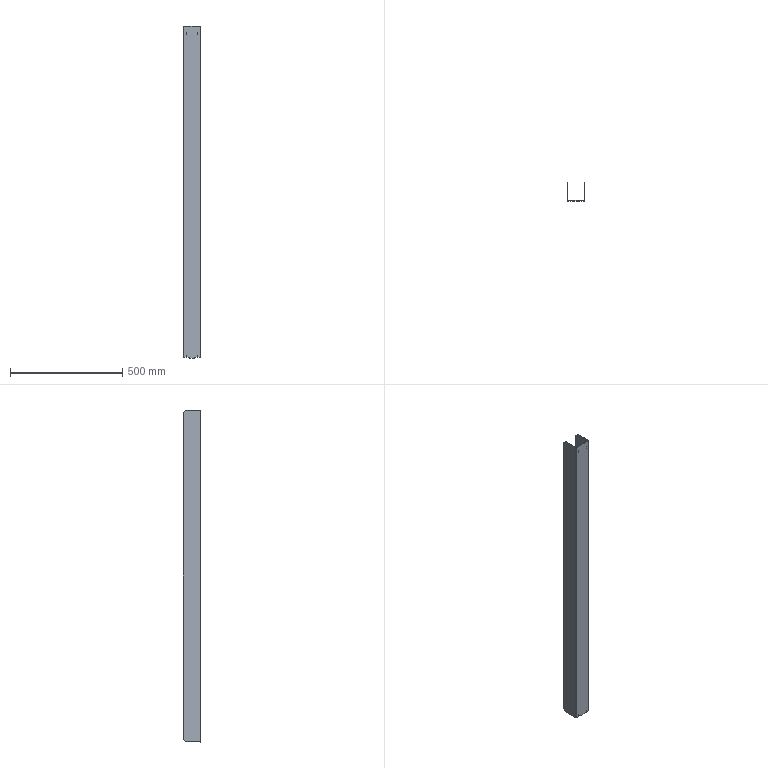Part | STEP file | SX-004-05 | 1 solid | 50 faces | box 80 x 80 x 1480 mm | volume 692801 mm3 | plane 46 | cylinder 4 | commonest cylinder face diameters 0.4 x2 4.4 x2